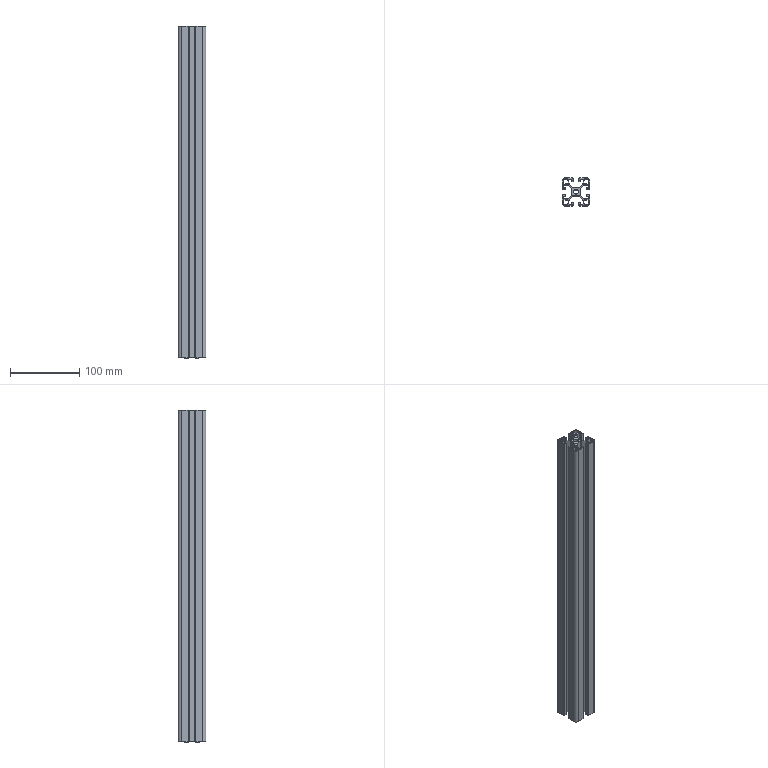Part | STEP file | LE-8-4040-S-OO_LE0314010444 | 1 solid | 188 faces | box 40 x 40 x 480 mm | volume 229559 mm3 | cylinder 94 | plane 94 | commonest cylinder face diameters 0.6 x30 2 x28 4 x16 0.4 x8 6 x4 9 x4